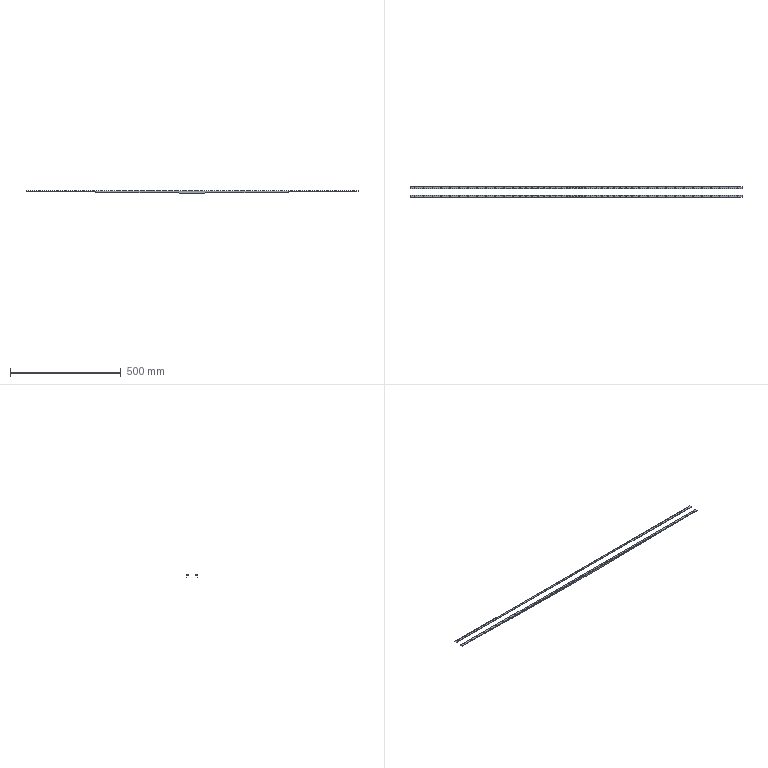Part | SolidWorks | features BaseBody 2 | 2 solids | 210 faces | box 1500 x 48 x 9.5 mm | volume 50625 mm3 | cylinder 190 | plane 20 | commonest cylinder face diameters 3.116 x96 3.2 x76 2.4 x16 1 x2